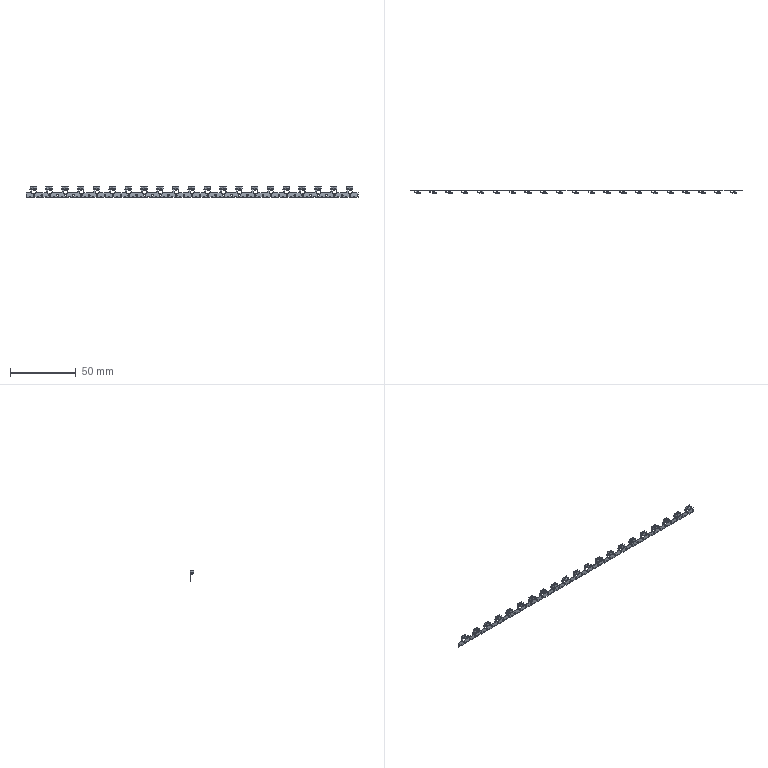Part | NX | 1 solid | 3621 faces | volume 334.675 mm3 | plane 2171 | cylinder 1156 | torus 252 | spline 42 | commonest cylinder face diameters 0.3 x336 0.2 x126 1.3 x106 0.5 x105 0.7 x105 0.35 x84